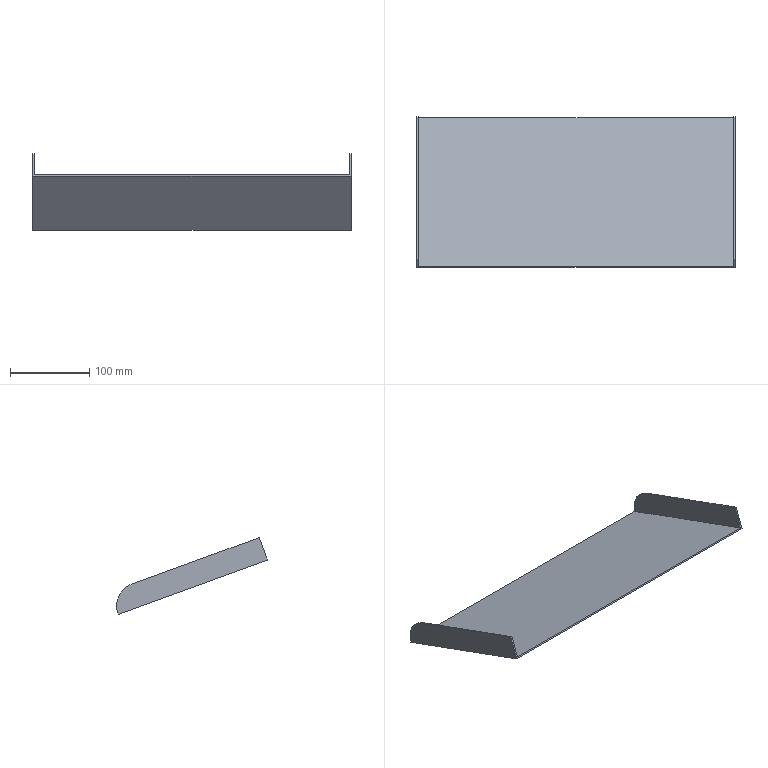Part | NX | features solid 2 | 1 solid | 12 faces | box 401.058 x 189.748 x 96.595 mm | volume 182051 mm3 | plane 10 | cylinder 2 | commonest cylinder face diameters 60 x2
STEP:
#1=CARTESIAN_POINT('',(835.942,1010.,-315.103));
#2=VERTEX_POINT('',#1);
#3=CARTESIAN_POINT('',(1233.,1010.,-315.103));
#4=VERTEX_POINT('',#3);
#5=CARTESIAN_POINT('',(845.942,1010.,-315.103));
#6=DIRECTION('',(-1.,0.,0.));
#7=VECTOR('',#6,1000.);
#8=LINE('',#5,#7);
#9=EDGE_CURVE('',#2,#4,#8,.F.);
#10=ORIENTED_EDGE('',*,*,#9,.T.);
#11=CARTESIAN_POINT('',(1233.,1197.876,-383.484));
#12=VERTEX_POINT('',#11);
#13=CARTESIAN_POINT('',(1233.,1038.191,-325.364));
#14=DIRECTION('',(0.,0.9397,-0.342));
#15=VECTOR('',#14,1000.);
#16=LINE('',#13,#15);
#17=EDGE_CURVE('',#4,#12,#16,.T.);
#18=ORIENTED_EDGE('',*,*,#17,.T.);
#19=CARTESIAN_POINT('',(1235.,1197.876,-383.484));
#20=VERTEX_POINT('',#19);
#21=CARTESIAN_POINT('',(1235.,1197.876,-383.484));
#22=CARTESIAN_POINT('',(1234.333,1197.876,-383.484));
#23=CARTESIAN_POINT('',(1233.667,1197.876,-383.484));
#24=CARTESIAN_POINT('',(1233.,1197.876,-383.484));
#25=B_SPLINE_CURVE_WITH_KNOTS('',3,(#21,#22,#23,#24),.UNSPECIFIED.,.F.,.F.,(4,4),(1310.704,1310.706),.UNSPECIFIED.);
#26=EDGE_CURVE('',#20,#12,#25,.T.);
#27=ORIENTED_EDGE('',*,*,#26,.F.);
#28=CARTESIAN_POINT('',(1235.,1197.939,-383.507));
#29=VERTEX_POINT('',#28);
#30=CARTESIAN_POINT('',(1235.,1038.191,-325.364));
#31=DIRECTION('',(0.,-0.9397,0.342));
#32=VECTOR('',#31,1000.);
#33=LINE('',#30,#32);
#34=EDGE_CURVE('',#20,#29,#33,.F.);
#35=ORIENTED_EDGE('',*,*,#34,.T.);
#36=CARTESIAN_POINT('',(833.942,1197.939,-383.507));
#37=VERTEX_POINT('',#36);
#38=CARTESIAN_POINT('',(845.942,1197.939,-383.507));
#39=DIRECTION('',(1.,0.,0.));
#40=VECTOR('',#39,1000.);
#41=LINE('',#38,#40);
#42=EDGE_CURVE('',#37,#29,#41,.T.);
#43=ORIENTED_EDGE('',*,*,#42,.F.);
#44=CARTESIAN_POINT('',(833.942,1197.876,-383.484));
#45=VERTEX_POINT('',#44);
#46=CARTESIAN_POINT('',(833.942,1038.191,-325.364));
#47=DIRECTION('',(0.,0.9397,-0.342));
#48=VECTOR('',#47,1000.);
#49=LINE('',#46,#48);
#50=EDGE_CURVE('',#45,#37,#49,.T.);
#51=ORIENTED_EDGE('',*,*,#50,.F.);
#52=CARTESIAN_POINT('',(835.942,1197.876,-383.484));
#53=VERTEX_POINT('',#52);
#54=CARTESIAN_POINT('',(835.942,1197.876,-383.484));
#55=CARTESIAN_POINT('',(835.275,1197.876,-383.484));
#56=CARTESIAN_POINT('',(834.608,1197.876,-383.484));
#57=CARTESIAN_POINT('',(833.942,1197.876,-383.484));
#58=B_SPLINE_CURVE_WITH_KNOTS('',3,(#54,#55,#56,#57),.UNSPECIFIED.,.F.,.F.,(4,4),(1310.699,1310.701),.UNSPECIFIED.);
#59=EDGE_CURVE('',#53,#45,#58,.T.);
#60=ORIENTED_EDGE('',*,*,#59,.F.);
#61=CARTESIAN_POINT('',(835.942,1038.191,-325.364));
#62=DIRECTION('',(0.,0.9397,-0.342));
#63=VECTOR('',#62,1000.);
#64=LINE('',#61,#63);
#65=EDGE_CURVE('',#2,#53,#64,.T.);
#66=ORIENTED_EDGE('',*,*,#65,.F.);
#67=EDGE_LOOP('',(#10,#18,#27,#35,#43,#51,#60,#66));
#68=FACE_BOUND('',#67,.T.);
#69=CARTESIAN_POINT('',(845.942,1038.191,-325.364));
#70=DIRECTION('',(0.,0.342,0.9397));
#71=DIRECTION('',(1.,0.,0.));
#72=AXIS2_PLACEMENT_3D('',#69,#70,#71);
#73=PLANE('',#72);
#74=ADVANCED_FACE('',(#68),#73,.T.);
#75=CARTESIAN_POINT('',(1235.,1019.577,-288.792));
#76=VERTEX_POINT('',#75);
#77=CARTESIAN_POINT('',(1235.,1009.316,-316.982));
#78=VERTEX_POINT('',#77);
#79=CARTESIAN_POINT('',(1235.,1010.,-315.103));
#80=DIRECTION('',(0.,-0.342,-0.9397));
#81=VECTOR('',#80,1000.);
#82=LINE('',#79,#81);
#83=EDGE_CURVE('',#76,#78,#82,.T.);
#84=ORIENTED_EDGE('',*,*,#83,.F.);
#85=CARTESIAN_POINT('',(1233.,1019.577,-288.792));
#86=VERTEX_POINT('',#85);
#87=CARTESIAN_POINT('',(1240.,1019.577,-288.792));
#88=DIRECTION('',(1.,0.,0.));
#89=VECTOR('',#88,1000.);
#90=LINE('',#87,#89);
#91=EDGE_CURVE('',#76,#86,#90,.F.);
#92=ORIENTED_EDGE('',*,*,#91,.T.);
#93=CARTESIAN_POINT('',(1233.,1009.316,-316.982));
#94=DIRECTION('',(0.,-0.342,-0.9397));
#95=VECTOR('',#94,1000.);
#96=LINE('',#93,#95);
#97=EDGE_CURVE('',#4,#86,#96,.F.);
#98=ORIENTED_EDGE('',*,*,#97,.F.);
#99=ORIENTED_EDGE('',*,*,#9,.F.);
#100=CARTESIAN_POINT('',(835.942,1019.577,-288.792));
#101=VERTEX_POINT('',#100);
#102=CARTESIAN_POINT('',(835.942,1009.316,-316.982));
#103=DIRECTION('',(0.,-0.342,-0.9397));
#104=VECTOR('',#103,1000.);
#105=LINE('',#102,#104);
#106=EDGE_CURVE('',#2,#101,#105,.F.);
#107=ORIENTED_EDGE('',*,*,#106,.T.);
#108=CARTESIAN_POINT('',(833.942,1019.577,-288.792));
#109=VERTEX_POINT('',#108);
#110=CARTESIAN_POINT('',(833.942,1019.577,-288.792));
#111=DIRECTION('',(1.,0.,0.));
#112=VECTOR('',#111,1000.);
#113=LINE('',#110,#112);
#114=EDGE_CURVE('',#109,#101,#113,.T.);
#115=ORIENTED_EDGE('',*,*,#114,.F.);
#116=CARTESIAN_POINT('',(833.942,1009.316,-316.982));
#117=VERTEX_POINT('',#116);
#118=CARTESIAN_POINT('',(833.942,1010.,-315.103));
#119=DIRECTION('',(0.,0.342,0.9397));
#120=VECTOR('',#119,1000.);
#121=LINE('',#118,#120);
#122=EDGE_CURVE('',#109,#117,#121,.F.);
#123=ORIENTED_EDGE('',*,*,#122,.T.);
#124=CARTESIAN_POINT('',(845.942,1009.316,-316.982));
#125=DIRECTION('',(-1.,0.,0.));
#126=VECTOR('',#125,1000.);
#127=LINE('',#124,#126);
#128=EDGE_CURVE('',#117,#78,#127,.F.);
#129=ORIENTED_EDGE('',*,*,#128,.T.);
#130=EDGE_LOOP('',(#84,#92,#98,#99,#107,#115,#123,#129));
#131=FACE_BOUND('',#130,.T.);
#132=CARTESIAN_POINT('',(845.942,1010.,-315.103));
#133=DIRECTION('',(0.,-0.9397,0.342));
#134=DIRECTION('',(1.,0.,0.));
#135=AXIS2_PLACEMENT_3D('',#132,#133,#134);
#136=PLANE('',#135);
#137=ADVANCED_FACE('',(#131),#136,.T.);
#138=ORIENTED_EDGE('',*,*,#34,.F.);
#139=CARTESIAN_POINT('',(1235.,1179.324,-346.935));
#140=VERTEX_POINT('',#139);
#141=CARTESIAN_POINT('',(1235.,1169.064,-375.126));
#142=DIRECTION('',(1.,0.,0.));
#143=DIRECTION('',(0.,0.,-1.));
#144=AXIS2_PLACEMENT_3D('',#141,#142,#143);
#145=CIRCLE('',#144,30.);
#146=EDGE_CURVE('',#20,#140,#145,.T.);
#147=ORIENTED_EDGE('',*,*,#146,.T.);
#148=CARTESIAN_POINT('',(1235.,1019.577,-288.792));
#149=DIRECTION('',(0.,-0.9397,0.342));
#150=VECTOR('',#149,1000.);
#151=LINE('',#148,#150);
#152=EDGE_CURVE('',#76,#140,#151,.F.);
#153=ORIENTED_EDGE('',*,*,#152,.F.);
#154=ORIENTED_EDGE('',*,*,#83,.T.);
#155=CARTESIAN_POINT('',(1235.,1197.254,-385.386));
#156=VERTEX_POINT('',#155);
#157=CARTESIAN_POINT('',(1235.,1037.507,-327.243));
#158=DIRECTION('',(0.,-0.9397,0.342));
#159=VECTOR('',#158,1000.);
#160=LINE('',#157,#159);
#161=EDGE_CURVE('',#78,#156,#160,.F.);
#162=ORIENTED_EDGE('',*,*,#161,.T.);
#163=CARTESIAN_POINT('',(1235.,1197.939,-383.507));
#164=DIRECTION('',(0.,0.342,0.9397));
#165=VECTOR('',#164,1000.);
#166=LINE('',#163,#165);
#167=EDGE_CURVE('',#29,#156,#166,.F.);
#168=ORIENTED_EDGE('',*,*,#167,.F.);
#169=EDGE_LOOP('',(#138,#147,#153,#154,#162,#168));
#170=FACE_BOUND('',#169,.T.);
#171=CARTESIAN_POINT('',(1235.,1038.191,-325.364));
#172=DIRECTION('',(1.,0.,0.));
#173=DIRECTION('',(0.,0.9397,-0.342));
#174=AXIS2_PLACEMENT_3D('',#171,#172,#173);
#175=PLANE('',#174);
#176=ADVANCED_FACE('',(#170),#175,.T.);
#177=ORIENTED_EDGE('',*,*,#167,.T.);
#178=CARTESIAN_POINT('',(833.942,1197.254,-385.386));
#179=VERTEX_POINT('',#178);
#180=CARTESIAN_POINT('',(845.942,1197.254,-385.386));
#181=DIRECTION('',(1.,0.,0.));
#182=VECTOR('',#181,1000.);
#183=LINE('',#180,#182);
#184=EDGE_CURVE('',#179,#156,#183,.T.);
#185=ORIENTED_EDGE('',*,*,#184,.F.);
#186=CARTESIAN_POINT('',(833.942,1197.939,-383.507));
#187=DIRECTION('',(0.,-0.342,-0.9397));
#188=VECTOR('',#187,1000.);
#189=LINE('',#186,#188);
#190=EDGE_CURVE('',#37,#179,#189,.T.);
#191=ORIENTED_EDGE('',*,*,#190,.F.);
#192=ORIENTED_EDGE('',*,*,#42,.T.);
#193=EDGE_LOOP('',(#177,#185,#191,#192));
#194=FACE_BOUND('',#193,.T.);
#195=CARTESIAN_POINT('',(845.942,1197.939,-383.507));
#196=DIRECTION('',(0.,-0.9397,0.342));
#197=DIRECTION('',(1.,0.,0.));
#198=AXIS2_PLACEMENT_3D('',#195,#196,#197);
#199=PLANE('',#198);
#200=ADVANCED_FACE('',(#194),#199,.F.);
#201=ORIENTED_EDGE('',*,*,#190,.T.);
#202=CARTESIAN_POINT('',(833.942,1037.507,-327.243));
#203=DIRECTION('',(0.,0.9397,-0.342));
#204=VECTOR('',#203,1000.);
#205=LINE('',#202,#204);
#206=EDGE_CURVE('',#117,#179,#205,.T.);
#207=ORIENTED_EDGE('',*,*,#206,.F.);
#208=ORIENTED_EDGE('',*,*,#122,.F.);
#209=CARTESIAN_POINT('',(833.942,1179.324,-346.935));
#210=VERTEX_POINT('',#209);
#211=CARTESIAN_POINT('',(833.942,1019.577,-288.792));
#212=DIRECTION('',(0.,0.9397,-0.342));
#213=VECTOR('',#212,1000.);
#214=LINE('',#211,#213);
#215=EDGE_CURVE('',#109,#210,#214,.T.);
#216=ORIENTED_EDGE('',*,*,#215,.T.);
#217=CARTESIAN_POINT('',(833.942,1169.064,-375.126));
#218=DIRECTION('',(1.,0.,0.));
#219=DIRECTION('',(0.,-0.342,-0.9397));
#220=AXIS2_PLACEMENT_3D('',#217,#218,#219);
#221=CIRCLE('',#220,30.);
#222=EDGE_CURVE('',#210,#45,#221,.F.);
#223=ORIENTED_EDGE('',*,*,#222,.T.);
#224=ORIENTED_EDGE('',*,*,#50,.T.);
#225=EDGE_LOOP('',(#201,#207,#208,#216,#223,#224));
#226=FACE_BOUND('',#225,.T.);
#227=CARTESIAN_POINT('',(833.942,1038.191,-325.364));
#228=DIRECTION('',(1.,0.,0.));
#229=DIRECTION('',(0.,0.9397,-0.342));
#230=AXIS2_PLACEMENT_3D('',#227,#228,#229);
#231=PLANE('',#230);
#232=ADVANCED_FACE('',(#226),#231,.F.);
#233=ORIENTED_EDGE('',*,*,#161,.F.);
#234=ORIENTED_EDGE('',*,*,#128,.F.);
#235=ORIENTED_EDGE('',*,*,#206,.T.);
#236=ORIENTED_EDGE('',*,*,#184,.T.);
#237=EDGE_LOOP('',(#233,#234,#235,#236));
#238=FACE_BOUND('',#237,.T.);
#239=CARTESIAN_POINT('',(845.942,1037.507,-327.243));
#240=DIRECTION('',(0.,0.342,0.9397));
#241=DIRECTION('',(1.,0.,0.));
#242=AXIS2_PLACEMENT_3D('',#239,#240,#241);
#243=PLANE('',#242);
#244=ADVANCED_FACE('',(#238),#243,.F.);
#245=CARTESIAN_POINT('',(835.942,1179.324,-346.935));
#246=VERTEX_POINT('',#245);
#247=CARTESIAN_POINT('',(835.942,1019.577,-288.792));
#248=DIRECTION('',(0.,0.9397,-0.342));
#249=VECTOR('',#248,1000.);
#250=LINE('',#247,#249);
#251=EDGE_CURVE('',#101,#246,#250,.T.);
#252=ORIENTED_EDGE('',*,*,#251,.T.);
#253=CARTESIAN_POINT('',(833.942,1179.324,-346.935));
#254=DIRECTION('',(1.,0.,0.));
#255=VECTOR('',#254,1000.);
#256=LINE('',#253,#255);
#257=EDGE_CURVE('',#246,#210,#256,.F.);
#258=ORIENTED_EDGE('',*,*,#257,.T.);
#259=ORIENTED_EDGE('',*,*,#215,.F.);
#260=ORIENTED_EDGE('',*,*,#114,.T.);
#261=EDGE_LOOP('',(#252,#258,#259,#260));
#262=FACE_BOUND('',#261,.T.);
#263=CARTESIAN_POINT('',(833.942,1019.577,-288.792));
#264=DIRECTION('',(0.,-0.342,-0.9397));
#265=DIRECTION('',(0.,0.9397,-0.342));
#266=AXIS2_PLACEMENT_3D('',#263,#264,#265);
#267=PLANE('',#266);
#268=ADVANCED_FACE('',(#262),#267,.F.);
#269=ORIENTED_EDGE('',*,*,#106,.F.);
#270=ORIENTED_EDGE('',*,*,#65,.T.);
#271=CARTESIAN_POINT('',(835.942,1169.064,-375.126));
#272=DIRECTION('',(1.,0.,0.));
#273=DIRECTION('',(0.,-0.342,-0.9397));
#274=AXIS2_PLACEMENT_3D('',#271,#272,#273);
#275=CIRCLE('',#274,30.);
#276=EDGE_CURVE('',#53,#246,#275,.T.);
#277=ORIENTED_EDGE('',*,*,#276,.T.);
#278=ORIENTED_EDGE('',*,*,#251,.F.);
#279=EDGE_LOOP('',(#269,#270,#277,#278));
#280=FACE_BOUND('',#279,.T.);
#281=CARTESIAN_POINT('',(835.942,1009.316,-316.982));
#282=DIRECTION('',(1.,0.,0.));
#283=DIRECTION('',(0.,-0.342,-0.9397));
#284=AXIS2_PLACEMENT_3D('',#281,#282,#283);
#285=PLANE('',#284);
#286=ADVANCED_FACE('',(#280),#285,.T.);
#287=ORIENTED_EDGE('',*,*,#276,.F.);
#288=ORIENTED_EDGE('',*,*,#59,.T.);
#289=ORIENTED_EDGE('',*,*,#222,.F.);
#290=ORIENTED_EDGE('',*,*,#257,.F.);
#291=EDGE_LOOP('',(#287,#288,#289,#290));
#292=FACE_BOUND('',#291,.T.);
#293=CARTESIAN_POINT('',(833.942,1169.064,-375.126));
#294=DIRECTION('',(-1.,0.,0.));
#295=DIRECTION('',(0.,0.342,0.9397));
#296=AXIS2_PLACEMENT_3D('',#293,#294,#295);
#297=CYLINDRICAL_SURFACE('',#296,30.);
#298=ADVANCED_FACE('',(#292),#297,.T.);
#299=ORIENTED_EDGE('',*,*,#152,.T.);
#300=CARTESIAN_POINT('',(1233.,1179.324,-346.935));
#301=VERTEX_POINT('',#300);
#302=CARTESIAN_POINT('',(1240.,1179.324,-346.935));
#303=DIRECTION('',(1.,0.,0.));
#304=VECTOR('',#303,1000.);
#305=LINE('',#302,#304);
#306=EDGE_CURVE('',#140,#301,#305,.F.);
#307=ORIENTED_EDGE('',*,*,#306,.T.);
#308=CARTESIAN_POINT('',(1233.,1019.577,-288.792));
#309=DIRECTION('',(0.,0.9397,-0.342));
#310=VECTOR('',#309,1000.);
#311=LINE('',#308,#310);
#312=EDGE_CURVE('',#86,#301,#311,.T.);
#313=ORIENTED_EDGE('',*,*,#312,.F.);
#314=ORIENTED_EDGE('',*,*,#91,.F.);
#315=EDGE_LOOP('',(#299,#307,#313,#314));
#316=FACE_BOUND('',#315,.T.);
#317=CARTESIAN_POINT('',(1240.,1019.577,-288.792));
#318=DIRECTION('',(0.,-0.342,-0.9397));
#319=DIRECTION('',(0.,0.9397,-0.342));
#320=AXIS2_PLACEMENT_3D('',#317,#318,#319);
#321=PLANE('',#320);
#322=ADVANCED_FACE('',(#316),#321,.F.);
#323=ORIENTED_EDGE('',*,*,#17,.F.);
#324=ORIENTED_EDGE('',*,*,#97,.T.);
#325=ORIENTED_EDGE('',*,*,#312,.T.);
#326=CARTESIAN_POINT('',(1233.,1169.064,-375.126));
#327=DIRECTION('',(1.,0.,0.));
#328=DIRECTION('',(0.,1.,0.));
#329=AXIS2_PLACEMENT_3D('',#326,#327,#328);
#330=CIRCLE('',#329,30.);
#331=EDGE_CURVE('',#301,#12,#330,.F.);
#332=ORIENTED_EDGE('',*,*,#331,.T.);
#333=EDGE_LOOP('',(#323,#324,#325,#332));
#334=FACE_BOUND('',#333,.T.);
#335=CARTESIAN_POINT('',(1233.,1009.316,-316.982));
#336=DIRECTION('',(1.,0.,0.));
#337=DIRECTION('',(0.,-0.342,-0.9397));
#338=AXIS2_PLACEMENT_3D('',#335,#336,#337);
#339=PLANE('',#338);
#340=ADVANCED_FACE('',(#334),#339,.F.);
#341=ORIENTED_EDGE('',*,*,#146,.F.);
#342=ORIENTED_EDGE('',*,*,#26,.T.);
#343=ORIENTED_EDGE('',*,*,#331,.F.);
#344=ORIENTED_EDGE('',*,*,#306,.F.);
#345=EDGE_LOOP('',(#341,#342,#343,#344));
#346=FACE_BOUND('',#345,.T.);
#347=CARTESIAN_POINT('',(1240.,1169.064,-375.126));
#348=DIRECTION('',(1.,0.,0.));
#349=DIRECTION('',(0.,-0.342,-0.9397));
#350=AXIS2_PLACEMENT_3D('',#347,#348,#349);
#351=CYLINDRICAL_SURFACE('',#350,30.);
#352=ADVANCED_FACE('',(#346),#351,.T.);
#353=CLOSED_SHELL('',(#74,#137,#176,#200,#232,#244,#268,#286,#298,#322,#340,#352));
#354=MANIFOLD_SOLID_BREP('',#353);
#355=(LENGTH_UNIT()NAMED_UNIT(*)SI_UNIT(.MILLI.,.METRE.));
#356=UNCERTAINTY_MEASURE_WITH_UNIT(LENGTH_MEASURE(0.0508),#355,'','');
#357=(NAMED_UNIT(*)PLANE_ANGLE_UNIT()SI_UNIT($,.RADIAN.));
#358=(NAMED_UNIT(*)SI_UNIT($,.STERADIAN.)SOLID_ANGLE_UNIT());
#359=(GEOMETRIC_REPRESENTATION_CONTEXT(3)GLOBAL_UNCERTAINTY_ASSIGNED_CONTEXT((#356))GLOBAL_UNIT_ASSIGNED_CONTEXT((#355,#357,#358))REPRESENTATION_CONTEXT('',''));
#360=ADVANCED_BREP_SHAPE_REPRESENTATION('',(#354),#359);